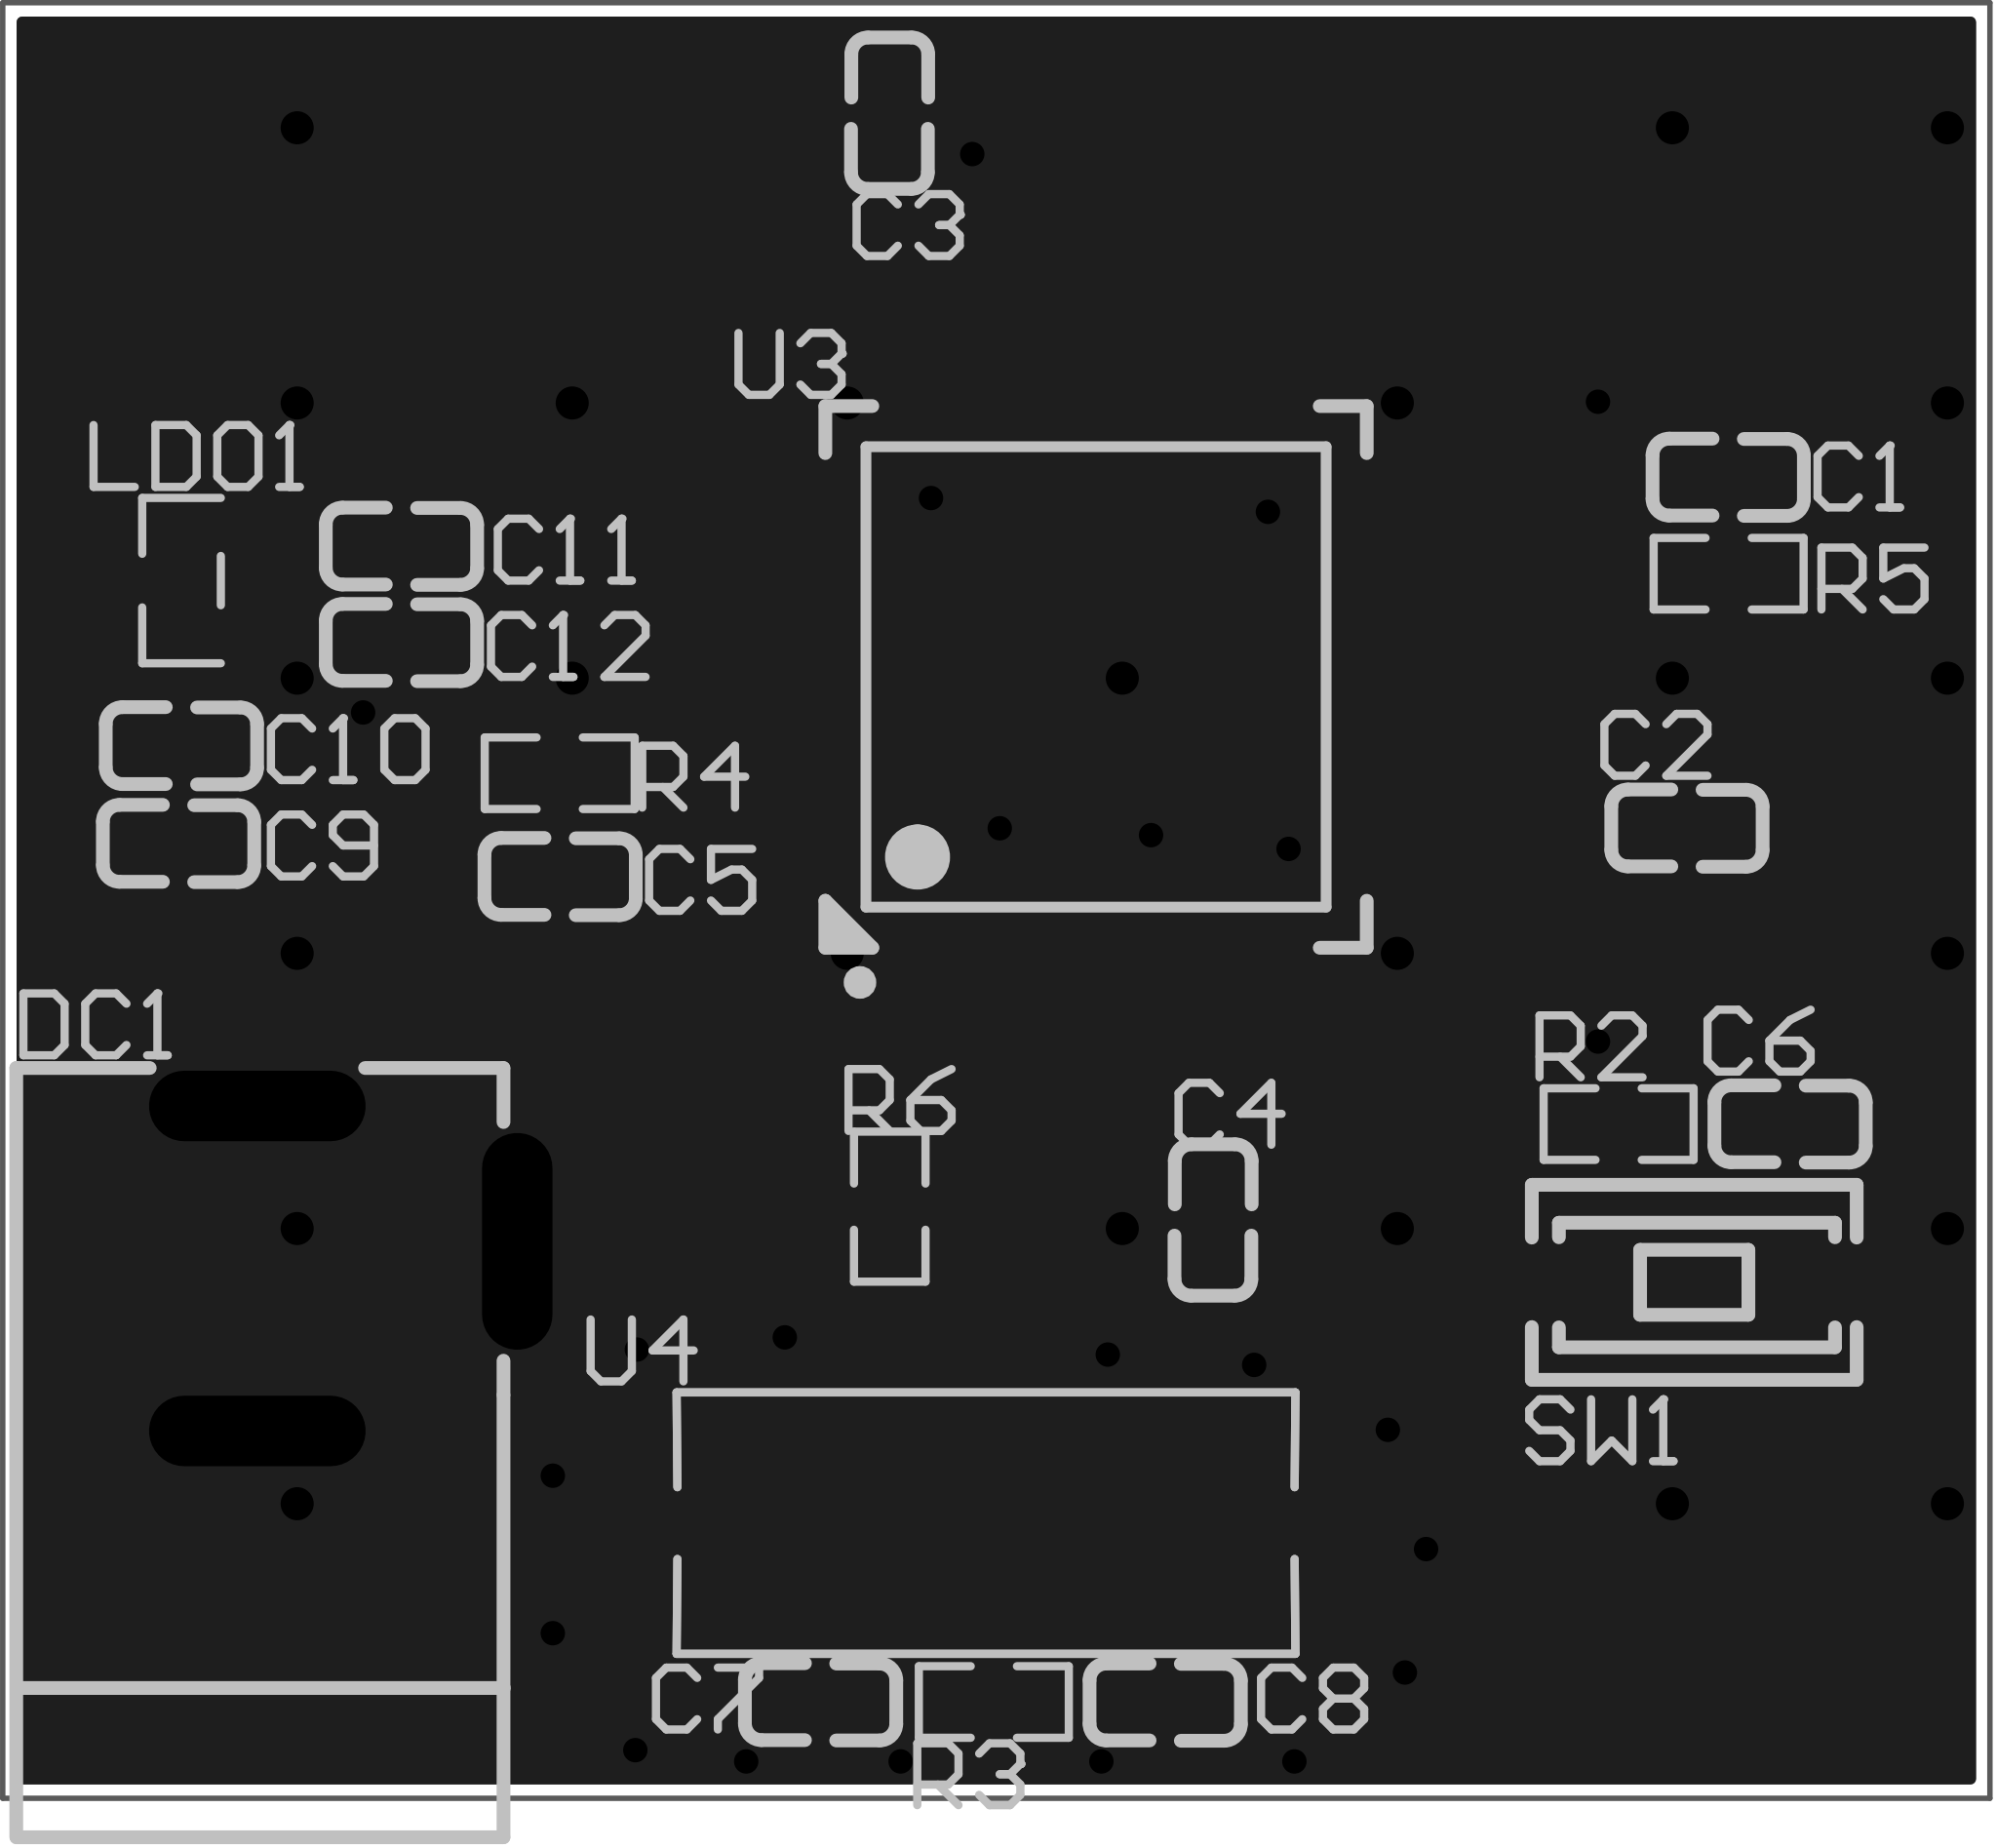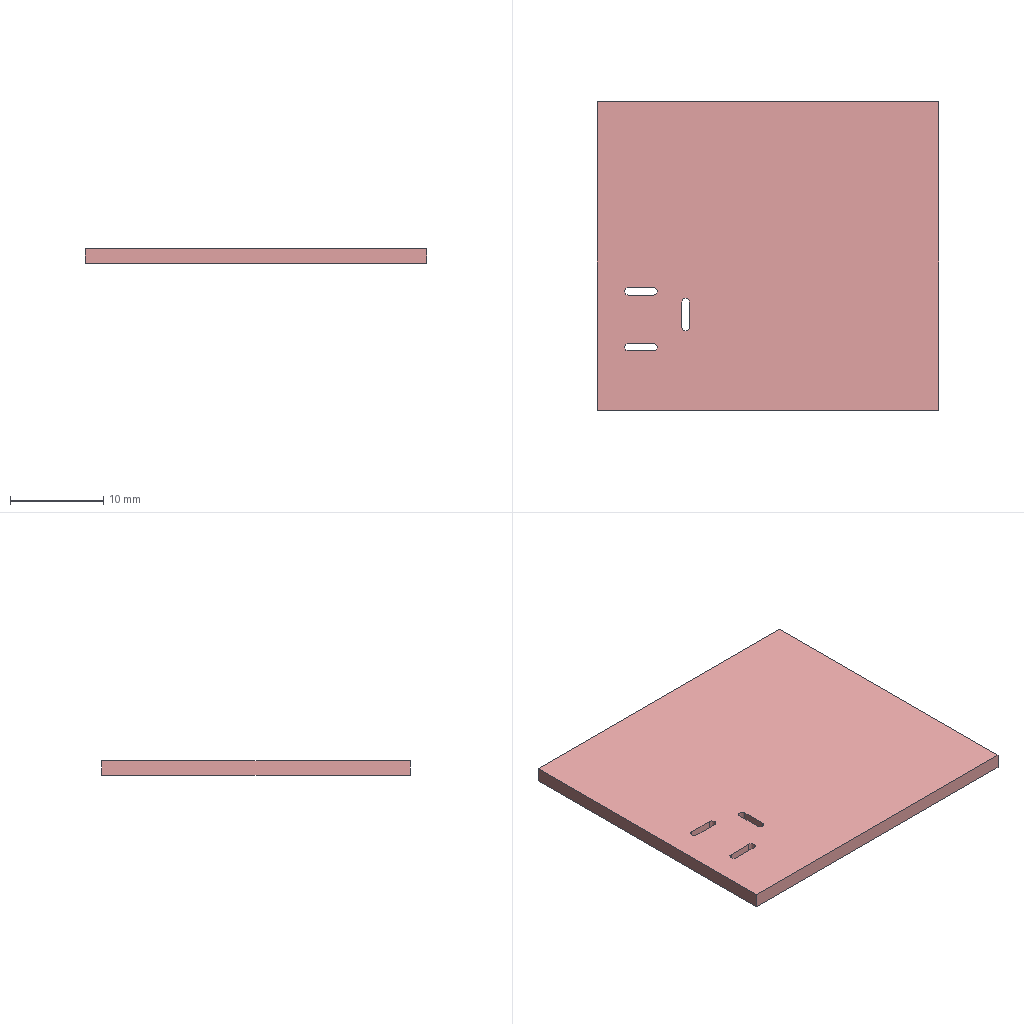Circuit board layout | Altium Designer | box 36.7 x 33.1 x 1.6 mm
Layer stack:
# Altium Designer layer stack of  (unit mm; dielectric type: 0 none, 1 core, 2 prepreg, 3 surface material)
index,name,kind,layer,copper_thickness_mm,dielectric_type,dielectric_thickness_mm,dielectric_material,dielectric_constant
0,Top Paste Mask Layer,other,,,,,,
1,Top Silkscreen Layer,other,,,,,,
2,Top Solder Mask Layer,dielectric,,,3,0.01,,3.3
3,Top Layer,copper,Top Layer,0.035,,,,
4,Dielectric1,dielectric,,,3,1.51,FR4,4.5
5,Bottom Layer,copper,Bottom Layer,0.035,,,,
6,Bottom Solder Mask Layer,dielectric,,,3,0.01,,3.3
7,Bottom Silkscreen Layer,other,,,,,,
8,Bottom Paste Mask Layer,other,,,,,,
# drill layer pairs: low layer,high layer
drill_pair,Top Layer,Bottom Layer
Part placement:
Designator,Comment,Layer,Footprint,Center-X(mm),Center-Y(mm),Rotation
C1,100nF,TopLayer,C0603,113.792,106.426,0
C2,100nF,TopLayer,C0603,113.03,99.949,0
C3,100nF,TopLayer,C0603,98.298,113.157,90
C4,100nF,TopLayer,C0603,104.267,92.71,270
C5,100nF,TopLayer,C0603,92.202,99.06,180
C6,100nF,TopLayer,C0603,114.935,94.488,0
C7,22pf,TopLayer,C0603,97.028,83.82,0
C8,22pf,TopLayer,C0603,103.378,83.82,180
C9,10uF,TopLayer,C0603,85.154,99.671,180
C10,100nF,TopLayer,C0603,85.207,101.475,180
C11,100nF,TopLayer,C0603,89.272,105.158,180
C12,10uF,TopLayer,C0603,89.272,103.38,180
DC1,,TopLayer,DC-2.0,89.017,91.823,270
LDO1,SC662K-3.3V,TopLayer,SOT-23-3_L2.9-W1.3-P1.90-LS2.4-BR,85.217,104.521,0
R2,10K,TopLayer,R0603,111.76,94.488,0
R3,1M,TopLayer,R0603,100.22,83.82,180
R4,0,TopLayer,R0603,92.202,100.965,180
R5,0,TopLayer,R0603,113.792,104.648,0
R6,0,TopLayer,R0603,98.298,92.964,90
SW1,SMD push button ANJIAN_2PIN,TopLayer,SW-SMD_L6.0-W3.6-LS8.0,113.157,91.567,0
U3,STM32F103RCT6TR,TopLayer,LQFP-64_L10.0-W10.0-P0.50-LS12.0-BL,102.108,102.743,0
U4,Crystal 8M-HC-49S/SMD,TopLayer,HC-49S_L11.4-W4.8-LS12.7,100.076,87.122,0
Pad and via stacks:
# Altium Designer via and pad stacks of  (unit mm). Each distinct definition once, with the count of objects using it.
# via: kind,start_layer,end_layer,hole_mm,diameter_mm,mode(0 simple;1 top-mid-bottom;2 full stack),diameter_per_layer,count,example_net
# pad: kind,layer,hole_mm,hole_type(0 round;1 square;2 slot),plating,top_size,top_shape(1 round;2 rect;3 octagon;9 rounded rect),mid_size,bottom_size,mode,footprint,size_per_layer,count,example
pad,Top Layer,0,0,plated,0.8x0.9,2,0.8x0.9,0.8x0.9,0,C0603,,24,C1.2
pad,Top Layer,0,0,plated,1.25x0.7,2,1.25x0.7,1.25x0.7,0,SOT-23-3_L2.9-W1.3-P1.90-LS2.4-BR,,3,LDO1.1
pad,Top Layer,0,0,plated,0.8065x0.864,2,0.8065x0.864,0.8065x0.864,0,R0603,,10,R2.2
pad,Top Layer,0,0,plated,1.5x1,2,1.5x1,1.5x1,0,SW-SMD_L6.0-W3.6-LS8.0,,2,SW1.1
pad,Top Layer,0,0,plated,2x0.3,1,2x0.3,2x0.3,0,LQFP-64_L10.0-W10.0-P0.50-LS12.0-BL,,32,U3.64
pad,Top Layer,0,0,plated,0.3x2,1,0.3x2,0.3x2,0,LQFP-64_L10.0-W10.0-P0.50-LS12.0-BL,,32,U3.48
pad,Top Layer,0,0,plated,5.5x1.3,2,5.5x1.3,5.5x1.3,0,HC-49S_L11.4-W4.8-LS12.7,,2,U4.2
pad,Multi-Layer,0.8001,2,plated,4x1.3,1,4x1.3,4x1.3,0,DC-2.0,,3,DC1.2
via,Top Layer,Bottom Layer,0.3048,0.45,0,,23,VCC
via,Top Layer,Bottom Layer,0.3048,0.61,0,,24,GND
Copper pours:
name,layer,net,type(0 solid;1 hatched;2 none)
Top Layer-GND,Top Layer,GND,0
Bottom Layer-GND,Bottom Layer,GND,0
Design rules, without the lines most boards share:
# Altium Designer design rules of  (exported by Altium Designer, unit mm)
# columns: name | kind | enabled | priority | scope1 | scope2 | descriptor | typed fields (field=value)
otherClearance | 52 | enabled | 1 | All | All | Hole To Hole Clearance (Gap=11.8mil) (All),(All) | gap=0.2997
viaSize | 11 | enabled | 1 | All | All | Routing Via (MinHoleWidth=11.811mil) (MaxHoleWidth=248.031mil) (PreferredHoleWidth=12.008mil) (MinWidth=17.717mil) (MaxWidth=393.701mil) (PreferedWidth=24.016mil) (All) | via_min_hole=0.3 via_max_hole=6.3 via_preferred_diameter=0.61 via_preferred_hole=0.305
solderMaskExpansion | 13 | enabled | 2 | All | All | Solder Mask Expansion (Expansion =2.008mil) (All) | expansion=0.051